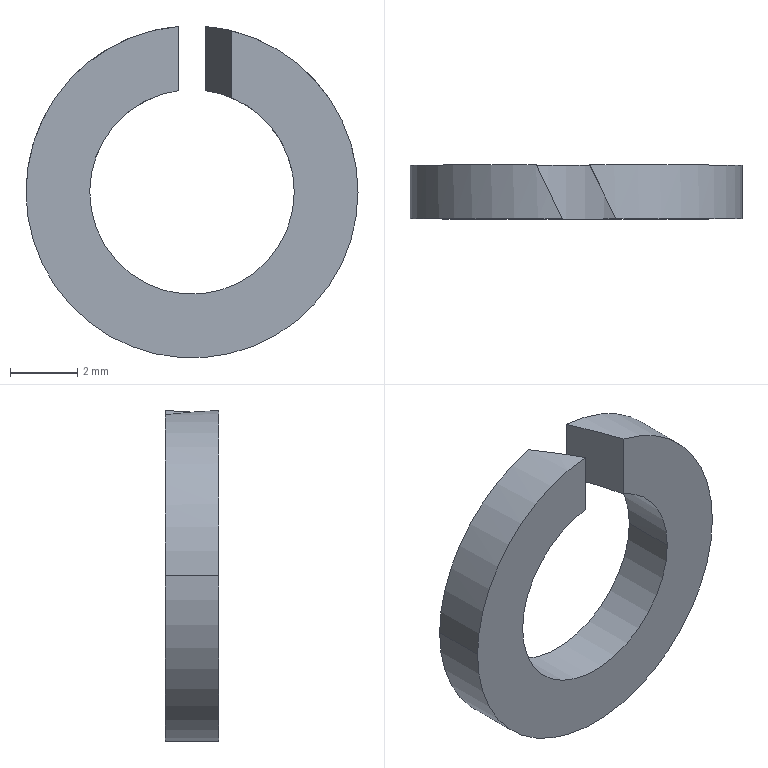Part | STEP file | WSPC-SUS-M6-1 | 1 solid | 10 faces | box 9.9 x 1.6 x 9.883 mm | volume 71.496 mm3 | cylinder 6 | plane 4 | commonest cylinder face diameters 6.1 x3 9.9 x3
STEP:
#1=CARTESIAN_POINT('',(3.05,1.6,-0.004612));
#2=VERTEX_POINT('',#1);
#3=CARTESIAN_POINT('',(0.4098,1.6,3.022));
#4=VERTEX_POINT('',#3);
#5=CARTESIAN_POINT('',(0.,1.6,0.));
#6=DIRECTION('',(0.,-1.,0.));
#7=DIRECTION('',(-1.,0.,0.001512));
#8=AXIS2_PLACEMENT_3D('',#5,#6,#7);
#9=CIRCLE('',#8,3.05);
#10=EDGE_CURVE('',#2,#4,#9,.T.);
#11=ORIENTED_EDGE('',*,*,#10,.F.);
#12=CARTESIAN_POINT('',(3.05,0.,-0.004612));
#13=VERTEX_POINT('',#12);
#14=CARTESIAN_POINT('',(3.05,1.6,-0.004612));
#15=DIRECTION('',(0.,-1.,0.));
#16=VECTOR('',#15,1000.);
#17=LINE('',#14,#16);
#18=EDGE_CURVE('',#2,#13,#17,.T.);
#19=ORIENTED_EDGE('',*,*,#18,.T.);
#20=CARTESIAN_POINT('',(1.19,0.,2.808));
#21=VERTEX_POINT('',#20);
#22=CARTESIAN_POINT('',(0.,0.,0.));
#23=DIRECTION('',(0.,1.,0.));
#24=DIRECTION('',(1.,0.,-0.001512));
#25=AXIS2_PLACEMENT_3D('',#22,#23,#24);
#26=CIRCLE('',#25,3.05);
#27=EDGE_CURVE('',#21,#13,#26,.T.);
#28=ORIENTED_EDGE('',*,*,#27,.F.);
#29=CARTESIAN_POINT('',(1.19,0.,2.808));
#30=CARTESIAN_POINT('',(0.9404,0.5122,2.914));
#31=CARTESIAN_POINT('',(0.6787,1.049,2.986));
#32=CARTESIAN_POINT('',(0.4098,1.6,3.022));
#33=(BOUNDED_CURVE()B_SPLINE_CURVE(3,(#29,#30,#31,#32),.UNSPECIFIED.,.F.,.F.)B_SPLINE_CURVE_WITH_KNOTS((4,4),(1.17,1.436),.UNSPECIFIED.)CURVE()GEOMETRIC_REPRESENTATION_ITEM()RATIONAL_B_SPLINE_CURVE((1.,0.9941,0.9941,1.))REPRESENTATION_ITEM(''));
#34=EDGE_CURVE('',#21,#4,#33,.T.);
#35=ORIENTED_EDGE('',*,*,#34,.T.);
#36=EDGE_LOOP('',(#11,#19,#28,#35));
#37=FACE_OUTER_BOUND('',#36,.T.);
#38=CARTESIAN_POINT('',(0.,1.6,0.));
#39=DIRECTION('',(0.,-1.,0.));
#40=DIRECTION('',(-1.,0.,0.001512));
#41=AXIS2_PLACEMENT_3D('',#38,#39,#40);
#42=CYLINDRICAL_SURFACE('',#41,3.05);
#43=ADVANCED_FACE('',(#37),#42,.F.);
#44=ORIENTED_EDGE('',*,*,#18,.F.);
#45=CARTESIAN_POINT('',(-3.05,1.6,0.004612));
#46=VERTEX_POINT('',#45);
#47=CARTESIAN_POINT('',(0.,1.6,0.));
#48=DIRECTION('',(0.,-1.,0.));
#49=DIRECTION('',(-1.,0.,0.001512));
#50=AXIS2_PLACEMENT_3D('',#47,#48,#49);
#51=CIRCLE('',#50,3.05);
#52=EDGE_CURVE('',#46,#2,#51,.T.);
#53=ORIENTED_EDGE('',*,*,#52,.F.);
#54=CARTESIAN_POINT('',(-3.05,0.,0.004612));
#55=VERTEX_POINT('',#54);
#56=CARTESIAN_POINT('',(-3.05,1.6,0.004612));
#57=DIRECTION('',(0.,-1.,0.));
#58=VECTOR('',#57,1000.);
#59=LINE('',#56,#58);
#60=EDGE_CURVE('',#46,#55,#59,.T.);
#61=ORIENTED_EDGE('',*,*,#60,.T.);
#62=CARTESIAN_POINT('',(0.,0.,0.));
#63=DIRECTION('',(0.,1.,0.));
#64=DIRECTION('',(1.,0.,-0.001512));
#65=AXIS2_PLACEMENT_3D('',#62,#63,#64);
#66=CIRCLE('',#65,3.05);
#67=EDGE_CURVE('',#13,#55,#66,.T.);
#68=ORIENTED_EDGE('',*,*,#67,.F.);
#69=EDGE_LOOP('',(#44,#53,#61,#68));
#70=FACE_OUTER_BOUND('',#69,.T.);
#71=CARTESIAN_POINT('',(0.,1.6,0.));
#72=DIRECTION('',(0.,-1.,0.));
#73=DIRECTION('',(-1.,0.,0.001512));
#74=AXIS2_PLACEMENT_3D('',#71,#72,#73);
#75=CYLINDRICAL_SURFACE('',#74,3.05);
#76=ADVANCED_FACE('',(#70),#75,.F.);
#77=CARTESIAN_POINT('',(-4.95,1.6,0.007486));
#78=VERTEX_POINT('',#77);
#79=CARTESIAN_POINT('',(4.95,1.6,-0.007486));
#80=VERTEX_POINT('',#79);
#81=CARTESIAN_POINT('',(0.,1.6,0.));
#82=DIRECTION('',(0.,-1.,0.));
#83=DIRECTION('',(-1.,0.,0.001512));
#84=AXIS2_PLACEMENT_3D('',#81,#82,#83);
#85=CIRCLE('',#84,4.95);
#86=EDGE_CURVE('',#78,#80,#85,.T.);
#87=ORIENTED_EDGE('',*,*,#86,.T.);
#88=CARTESIAN_POINT('',(4.95,0.,-0.007486));
#89=VERTEX_POINT('',#88);
#90=CARTESIAN_POINT('',(4.95,1.6,-0.007486));
#91=DIRECTION('',(0.,-1.,0.));
#92=VECTOR('',#91,1000.);
#93=LINE('',#90,#92);
#94=EDGE_CURVE('',#80,#89,#93,.T.);
#95=ORIENTED_EDGE('',*,*,#94,.T.);
#96=CARTESIAN_POINT('',(-4.95,0.,0.007486));
#97=VERTEX_POINT('',#96);
#98=CARTESIAN_POINT('',(0.,0.,0.));
#99=DIRECTION('',(0.,1.,0.));
#100=DIRECTION('',(1.,0.,-0.001512));
#101=AXIS2_PLACEMENT_3D('',#98,#99,#100);
#102=CIRCLE('',#101,4.95);
#103=EDGE_CURVE('',#89,#97,#102,.T.);
#104=ORIENTED_EDGE('',*,*,#103,.T.);
#105=CARTESIAN_POINT('',(-4.95,1.6,0.007486));
#106=DIRECTION('',(0.,-1.,0.));
#107=VECTOR('',#106,1000.);
#108=LINE('',#105,#107);
#109=EDGE_CURVE('',#78,#97,#108,.T.);
#110=ORIENTED_EDGE('',*,*,#109,.F.);
#111=EDGE_LOOP('',(#87,#95,#104,#110));
#112=FACE_OUTER_BOUND('',#111,.T.);
#113=CARTESIAN_POINT('',(0.,1.6,0.));
#114=DIRECTION('',(0.,-1.,0.));
#115=DIRECTION('',(-1.,0.,0.001512));
#116=AXIS2_PLACEMENT_3D('',#113,#114,#115);
#117=CYLINDRICAL_SURFACE('',#116,4.95);
#118=ADVANCED_FACE('',(#112),#117,.T.);
#119=CARTESIAN_POINT('',(-1.19,1.6,4.805));
#120=VERTEX_POINT('',#119);
#121=CARTESIAN_POINT('',(0.,1.6,0.));
#122=DIRECTION('',(0.,-1.,0.));
#123=DIRECTION('',(-1.,0.,0.001512));
#124=AXIS2_PLACEMENT_3D('',#121,#122,#123);
#125=CIRCLE('',#124,4.95);
#126=EDGE_CURVE('',#120,#78,#125,.T.);
#127=ORIENTED_EDGE('',*,*,#126,.T.);
#128=ORIENTED_EDGE('',*,*,#109,.T.);
#129=CARTESIAN_POINT('',(-0.4098,0.,4.933));
#130=VERTEX_POINT('',#129);
#131=CARTESIAN_POINT('',(0.,0.,0.));
#132=DIRECTION('',(0.,1.,0.));
#133=DIRECTION('',(1.,0.,-0.001512));
#134=AXIS2_PLACEMENT_3D('',#131,#132,#133);
#135=CIRCLE('',#134,4.95);
#136=EDGE_CURVE('',#97,#130,#135,.T.);
#137=ORIENTED_EDGE('',*,*,#136,.T.);
#138=CARTESIAN_POINT('',(-0.4098,0.,4.933));
#139=CARTESIAN_POINT('',(-0.6731,0.5398,4.911));
#140=CARTESIAN_POINT('',(-0.9338,1.074,4.868));
#141=CARTESIAN_POINT('',(-1.19,1.6,4.805));
#142=(BOUNDED_CURVE()B_SPLINE_CURVE(3,(#138,#139,#140,#141),.UNSPECIFIED.,.F.,.F.)B_SPLINE_CURVE_WITH_KNOTS((4,4),(1.654,1.814),.UNSPECIFIED.)CURVE()GEOMETRIC_REPRESENTATION_ITEM()RATIONAL_B_SPLINE_CURVE((1.,0.9979,0.9979,1.))REPRESENTATION_ITEM(''));
#143=EDGE_CURVE('',#130,#120,#142,.T.);
#144=ORIENTED_EDGE('',*,*,#143,.T.);
#145=EDGE_LOOP('',(#127,#128,#137,#144));
#146=FACE_OUTER_BOUND('',#145,.T.);
#147=CARTESIAN_POINT('',(0.,1.6,0.));
#148=DIRECTION('',(0.,-1.,0.));
#149=DIRECTION('',(-1.,0.,0.001512));
#150=AXIS2_PLACEMENT_3D('',#147,#148,#149);
#151=CYLINDRICAL_SURFACE('',#150,4.95);
#152=ADVANCED_FACE('',(#146),#151,.T.);
#153=CARTESIAN_POINT('',(-0.4098,0.,3.022));
#154=VERTEX_POINT('',#153);
#155=CARTESIAN_POINT('',(-0.4098,0.,4.95));
#156=DIRECTION('',(0.,0.,-1.));
#157=VECTOR('',#156,1000.);
#158=LINE('',#155,#157);
#159=EDGE_CURVE('',#130,#154,#158,.T.);
#160=ORIENTED_EDGE('',*,*,#159,.F.);
#161=ORIENTED_EDGE('',*,*,#136,.F.);
#162=ORIENTED_EDGE('',*,*,#103,.F.);
#163=CARTESIAN_POINT('',(1.19,0.,4.805));
#164=VERTEX_POINT('',#163);
#165=CARTESIAN_POINT('',(0.,0.,0.));
#166=DIRECTION('',(0.,1.,0.));
#167=DIRECTION('',(1.,0.,-0.001512));
#168=AXIS2_PLACEMENT_3D('',#165,#166,#167);
#169=CIRCLE('',#168,4.95);
#170=EDGE_CURVE('',#164,#89,#169,.T.);
#171=ORIENTED_EDGE('',*,*,#170,.F.);
#172=CARTESIAN_POINT('',(1.19,0.,4.95));
#173=DIRECTION('',(0.,0.,-1.));
#174=VECTOR('',#173,1000.);
#175=LINE('',#172,#174);
#176=EDGE_CURVE('',#164,#21,#175,.T.);
#177=ORIENTED_EDGE('',*,*,#176,.T.);
#178=ORIENTED_EDGE('',*,*,#27,.T.);
#179=ORIENTED_EDGE('',*,*,#67,.T.);
#180=CARTESIAN_POINT('',(0.,0.,0.));
#181=DIRECTION('',(0.,1.,0.));
#182=DIRECTION('',(1.,0.,-0.001512));
#183=AXIS2_PLACEMENT_3D('',#180,#181,#182);
#184=CIRCLE('',#183,3.05);
#185=EDGE_CURVE('',#55,#154,#184,.T.);
#186=ORIENTED_EDGE('',*,*,#185,.T.);
#187=EDGE_LOOP('',(#160,#161,#162,#171,#177,#178,#179,#186));
#188=FACE_OUTER_BOUND('',#187,.T.);
#189=CARTESIAN_POINT('',(0.,0.,0.));
#190=DIRECTION('',(0.,-1.,0.));
#191=DIRECTION('',(-1.,0.,0.001512));
#192=AXIS2_PLACEMENT_3D('',#189,#190,#191);
#193=PLANE('',#192);
#194=ADVANCED_FACE('',(#188),#193,.T.);
#195=CARTESIAN_POINT('',(0.4098,1.6,4.933));
#196=VERTEX_POINT('',#195);
#197=CARTESIAN_POINT('',(0.4098,1.6,4.95));
#198=DIRECTION('',(0.,0.,-1.));
#199=VECTOR('',#198,1000.);
#200=LINE('',#197,#199);
#201=EDGE_CURVE('',#196,#4,#200,.T.);
#202=ORIENTED_EDGE('',*,*,#201,.F.);
#203=CARTESIAN_POINT('',(0.,1.6,0.));
#204=DIRECTION('',(0.,-1.,0.));
#205=DIRECTION('',(-1.,0.,0.001512));
#206=AXIS2_PLACEMENT_3D('',#203,#204,#205);
#207=CIRCLE('',#206,4.95);
#208=EDGE_CURVE('',#80,#196,#207,.T.);
#209=ORIENTED_EDGE('',*,*,#208,.F.);
#210=ORIENTED_EDGE('',*,*,#86,.F.);
#211=ORIENTED_EDGE('',*,*,#126,.F.);
#212=CARTESIAN_POINT('',(-1.19,1.6,2.808));
#213=VERTEX_POINT('',#212);
#214=CARTESIAN_POINT('',(-1.19,1.6,4.95));
#215=DIRECTION('',(0.,0.,-1.));
#216=VECTOR('',#215,1000.);
#217=LINE('',#214,#216);
#218=EDGE_CURVE('',#120,#213,#217,.T.);
#219=ORIENTED_EDGE('',*,*,#218,.T.);
#220=CARTESIAN_POINT('',(0.,1.6,0.));
#221=DIRECTION('',(0.,-1.,0.));
#222=DIRECTION('',(-1.,0.,0.001512));
#223=AXIS2_PLACEMENT_3D('',#220,#221,#222);
#224=CIRCLE('',#223,3.05);
#225=EDGE_CURVE('',#213,#46,#224,.T.);
#226=ORIENTED_EDGE('',*,*,#225,.T.);
#227=ORIENTED_EDGE('',*,*,#52,.T.);
#228=ORIENTED_EDGE('',*,*,#10,.T.);
#229=EDGE_LOOP('',(#202,#209,#210,#211,#219,#226,#227,#228));
#230=FACE_OUTER_BOUND('',#229,.T.);
#231=CARTESIAN_POINT('',(0.,1.6,0.));
#232=DIRECTION('',(0.,1.,0.));
#233=DIRECTION('',(1.,0.,-0.001512));
#234=AXIS2_PLACEMENT_3D('',#231,#232,#233);
#235=PLANE('',#234);
#236=ADVANCED_FACE('',(#230),#235,.T.);
#237=ORIENTED_EDGE('',*,*,#94,.F.);
#238=ORIENTED_EDGE('',*,*,#208,.T.);
#239=CARTESIAN_POINT('',(0.4098,1.6,4.933));
#240=CARTESIAN_POINT('',(0.6731,1.06,4.911));
#241=CARTESIAN_POINT('',(0.9338,0.5257,4.868));
#242=CARTESIAN_POINT('',(1.19,0.,4.805));
#243=(BOUNDED_CURVE()B_SPLINE_CURVE(3,(#239,#240,#241,#242),.UNSPECIFIED.,.F.,.F.)B_SPLINE_CURVE_WITH_KNOTS((4,4),(4.795,4.955),.UNSPECIFIED.)CURVE()GEOMETRIC_REPRESENTATION_ITEM()RATIONAL_B_SPLINE_CURVE((1.,0.9979,0.9979,1.))REPRESENTATION_ITEM(''));
#244=EDGE_CURVE('',#196,#164,#243,.T.);
#245=ORIENTED_EDGE('',*,*,#244,.T.);
#246=ORIENTED_EDGE('',*,*,#170,.T.);
#247=EDGE_LOOP('',(#237,#238,#245,#246));
#248=FACE_OUTER_BOUND('',#247,.T.);
#249=CARTESIAN_POINT('',(0.,1.6,0.));
#250=DIRECTION('',(0.,-1.,0.));
#251=DIRECTION('',(-1.,0.,0.001512));
#252=AXIS2_PLACEMENT_3D('',#249,#250,#251);
#253=CYLINDRICAL_SURFACE('',#252,4.95);
#254=ADVANCED_FACE('',(#248),#253,.T.);
#255=ORIENTED_EDGE('',*,*,#201,.T.);
#256=ORIENTED_EDGE('',*,*,#34,.F.);
#257=ORIENTED_EDGE('',*,*,#176,.F.);
#258=ORIENTED_EDGE('',*,*,#244,.F.);
#259=EDGE_LOOP('',(#255,#256,#257,#258));
#260=FACE_OUTER_BOUND('',#259,.T.);
#261=CARTESIAN_POINT('',(1.19,0.,4.95));
#262=DIRECTION('',(-0.8988,-0.4384,0.));
#263=DIRECTION('',(0.4384,-0.8988,0.));
#264=AXIS2_PLACEMENT_3D('',#261,#262,#263);
#265=PLANE('',#264);
#266=ADVANCED_FACE('',(#260),#265,.T.);
#267=ORIENTED_EDGE('',*,*,#159,.T.);
#268=CARTESIAN_POINT('',(-1.19,1.6,2.808));
#269=CARTESIAN_POINT('',(-0.9404,1.088,2.914));
#270=CARTESIAN_POINT('',(-0.6787,0.5513,2.986));
#271=CARTESIAN_POINT('',(-0.4098,0.,3.022));
#272=(BOUNDED_CURVE()B_SPLINE_CURVE(3,(#268,#269,#270,#271),.UNSPECIFIED.,.F.,.F.)B_SPLINE_CURVE_WITH_KNOTS((4,4),(4.312,4.578),.UNSPECIFIED.)CURVE()GEOMETRIC_REPRESENTATION_ITEM()RATIONAL_B_SPLINE_CURVE((1.,0.9941,0.9941,1.))REPRESENTATION_ITEM(''));
#273=EDGE_CURVE('',#213,#154,#272,.T.);
#274=ORIENTED_EDGE('',*,*,#273,.F.);
#275=ORIENTED_EDGE('',*,*,#218,.F.);
#276=ORIENTED_EDGE('',*,*,#143,.F.);
#277=EDGE_LOOP('',(#267,#274,#275,#276));
#278=FACE_OUTER_BOUND('',#277,.T.);
#279=CARTESIAN_POINT('',(-1.19,1.6,4.95));
#280=DIRECTION('',(0.8988,0.4384,0.));
#281=DIRECTION('',(-0.4384,0.8988,0.));
#282=AXIS2_PLACEMENT_3D('',#279,#280,#281);
#283=PLANE('',#282);
#284=ADVANCED_FACE('',(#278),#283,.T.);
#285=ORIENTED_EDGE('',*,*,#60,.F.);
#286=ORIENTED_EDGE('',*,*,#225,.F.);
#287=ORIENTED_EDGE('',*,*,#273,.T.);
#288=ORIENTED_EDGE('',*,*,#185,.F.);
#289=EDGE_LOOP('',(#285,#286,#287,#288));
#290=FACE_OUTER_BOUND('',#289,.T.);
#291=CARTESIAN_POINT('',(0.,1.6,0.));
#292=DIRECTION('',(0.,-1.,0.));
#293=DIRECTION('',(-1.,0.,0.001512));
#294=AXIS2_PLACEMENT_3D('',#291,#292,#293);
#295=CYLINDRICAL_SURFACE('',#294,3.05);
#296=ADVANCED_FACE('',(#290),#295,.F.);
#297=CLOSED_SHELL('',(#43,#76,#118,#152,#194,#236,#254,#266,#284,#296));
#298=MANIFOLD_SOLID_BREP('',#297);
#299=CARTESIAN_POINT('',(0.,0.,0.));
#300=DIRECTION('',(0.,0.,1.));
#301=DIRECTION('',(1.,0.,0.));
#302=AXIS2_PLACEMENT_3D('',#299,#300,#301);
#303=(LENGTH_UNIT()NAMED_UNIT(*)SI_UNIT(.MILLI.,.METRE.));
#304=UNCERTAINTY_MEASURE_WITH_UNIT(LENGTH_MEASURE(0.00001),#303,'','');
#305=(NAMED_UNIT(*)PLANE_ANGLE_UNIT()SI_UNIT($,.RADIAN.));
#306=(NAMED_UNIT(*)SI_UNIT($,.STERADIAN.)SOLID_ANGLE_UNIT());
#307=(GEOMETRIC_REPRESENTATION_CONTEXT(3)GLOBAL_UNCERTAINTY_ASSIGNED_CONTEXT((#304))GLOBAL_UNIT_ASSIGNED_CONTEXT((#303,#305,#306))REPRESENTATION_CONTEXT('',''));
#308=ADVANCED_BREP_SHAPE_REPRESENTATION('',(#298,#302),#307);